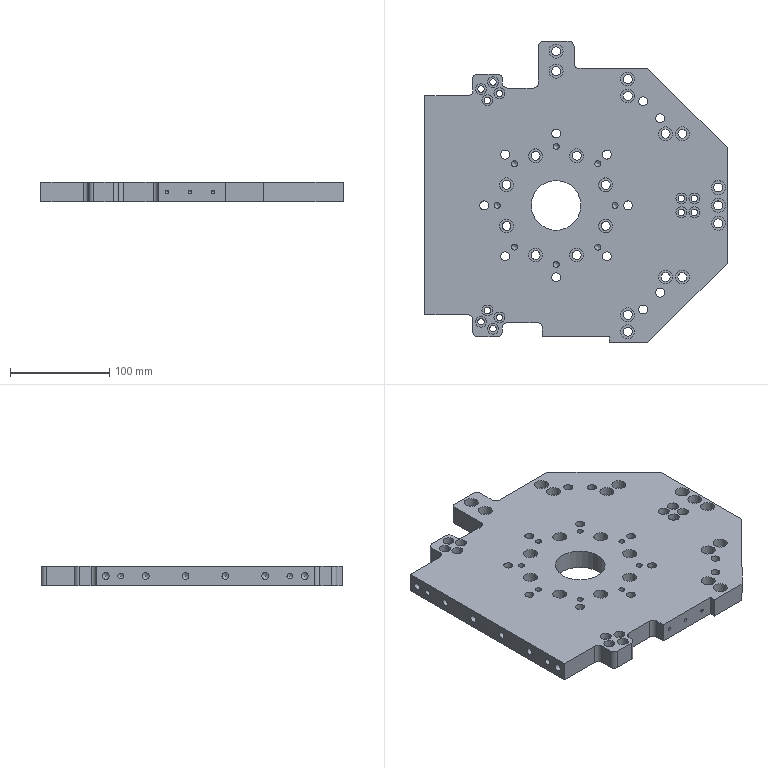Part | 1 solid | 211 faces | box 304 x 303 x 20 mm | volume 1335009 mm3 | cylinder 123 | plane 69 | cone 19 | commonest cylinder face diameters 9 x33 14 x33 10 x13 6.6 x12 11 x12 6 x10